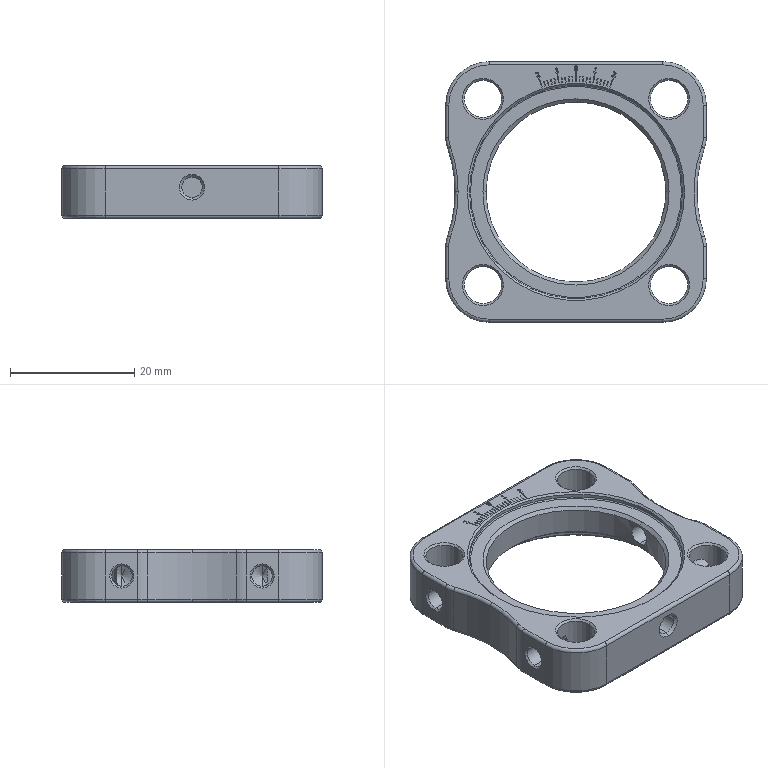Part | STEP file | 1 solid | 314 faces | box 42 x 42 x 8.5 mm | volume 6481 mm3 | plane 145 | cylinder 51 | spline 48 | cone 44 | torus 26 | commonest cylinder face diameters 1 x12 3.3 x12 6 x8 10 x4 14 x4 34.4 x4